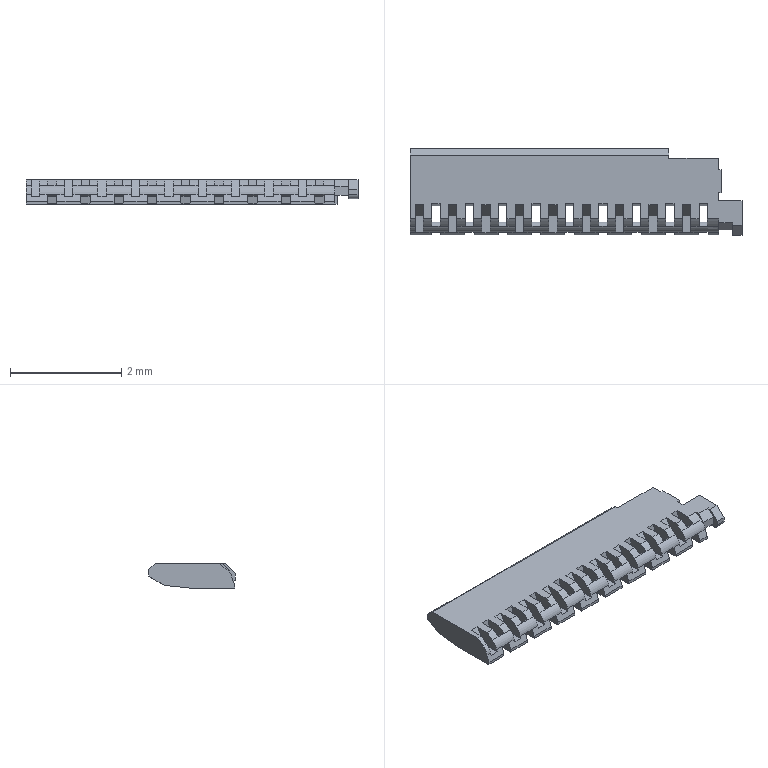Part | Creo | 1 solid | 193 faces | box 5.96 x 1.56 x 0.4431 mm | volume 2.904 mm3 | plane 154 | cylinder 39 | commonest cylinder face diameters 1.165 x19 0.39 x10 0.2 x9 0.16 x1